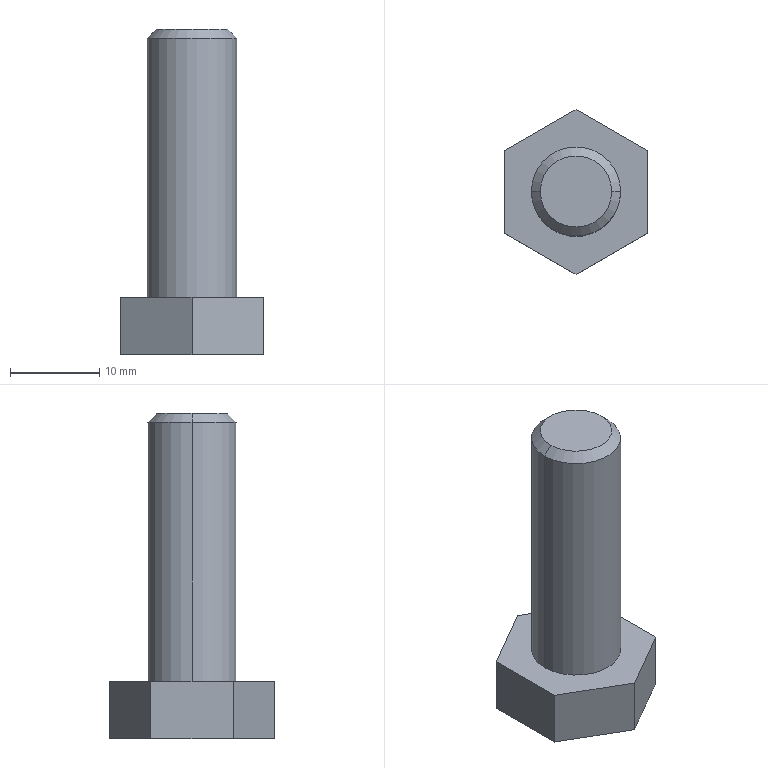Part | SolidWorks | features Chamfer 1, Extrusion 1, ICE 1, RefAxis 1 | 1 solid | 13 faces | box 16 x 18.475 x 36.4 mm | volume 3760 mm3 | plane 9 | cone 2 | cylinder 2 | commonest cylinder face diameters 10 x2
STEP:
#1=CARTESIAN_POINT('',(4.,0.,36.4));
#2=VERTEX_POINT('',#1);
#3=CARTESIAN_POINT('',(-4.,0.,36.4));
#4=VERTEX_POINT('',#3);
#5=CARTESIAN_POINT('',(0.,0.,36.4));
#6=DIRECTION('',(0.,0.,1.));
#7=DIRECTION('',(1.,0.,0.));
#8=AXIS2_PLACEMENT_3D('',#5,#6,#7);
#9=CIRCLE('',#8,4.);
#10=EDGE_CURVE('',#2,#4,#9,.T.);
#11=ORIENTED_EDGE('',*,*,#10,.F.);
#12=CARTESIAN_POINT('',(5.,0.,35.4));
#13=VERTEX_POINT('',#12);
#14=CARTESIAN_POINT('',(4.,0.,36.4));
#15=DIRECTION('',(0.7071,0.,-0.7071));
#16=VECTOR('',#15,1000.);
#17=LINE('',#14,#16);
#18=EDGE_CURVE('',#2,#13,#17,.T.);
#19=ORIENTED_EDGE('',*,*,#18,.T.);
#20=CARTESIAN_POINT('',(-5.,0.,35.4));
#21=VERTEX_POINT('',#20);
#22=CARTESIAN_POINT('',(0.,0.,35.4));
#23=DIRECTION('',(0.,0.,-1.));
#24=DIRECTION('',(1.,0.,0.));
#25=AXIS2_PLACEMENT_3D('',#22,#23,#24);
#26=CIRCLE('',#25,5.);
#27=EDGE_CURVE('',#21,#13,#26,.T.);
#28=ORIENTED_EDGE('',*,*,#27,.F.);
#29=CARTESIAN_POINT('',(-4.,0.,36.4));
#30=DIRECTION('',(-0.7071,0.,-0.7071));
#31=VECTOR('',#30,1000.);
#32=LINE('',#29,#31);
#33=EDGE_CURVE('',#4,#21,#32,.T.);
#34=ORIENTED_EDGE('',*,*,#33,.F.);
#35=EDGE_LOOP('',(#11,#19,#28,#34));
#36=FACE_OUTER_BOUND('',#35,.T.);
#37=CARTESIAN_POINT('',(0.,0.,36.4));
#38=DIRECTION('',(0.,0.,-1.));
#39=DIRECTION('',(-1.,0.,0.));
#40=AXIS2_PLACEMENT_3D('',#37,#38,#39);
#41=CONICAL_SURFACE('',#40,4.,0.7854);
#42=ADVANCED_FACE('',(#36),#41,.T.);
#43=ORIENTED_EDGE('',*,*,#27,.T.);
#44=CARTESIAN_POINT('',(5.,0.,6.4));
#45=VERTEX_POINT('',#44);
#46=CARTESIAN_POINT('',(5.,0.,36.4));
#47=DIRECTION('',(0.,0.,-1.));
#48=VECTOR('',#47,1000.);
#49=LINE('',#46,#48);
#50=EDGE_CURVE('',#13,#45,#49,.T.);
#51=ORIENTED_EDGE('',*,*,#50,.T.);
#52=CARTESIAN_POINT('',(-5.,0.,6.4));
#53=VERTEX_POINT('',#52);
#54=CARTESIAN_POINT('',(0.,0.,6.4));
#55=DIRECTION('',(0.,0.,1.));
#56=DIRECTION('',(1.,0.,0.));
#57=AXIS2_PLACEMENT_3D('',#54,#55,#56);
#58=CIRCLE('',#57,5.);
#59=EDGE_CURVE('',#45,#53,#58,.T.);
#60=ORIENTED_EDGE('',*,*,#59,.T.);
#61=CARTESIAN_POINT('',(-5.,0.,36.4));
#62=DIRECTION('',(0.,0.,-1.));
#63=VECTOR('',#62,1000.);
#64=LINE('',#61,#63);
#65=EDGE_CURVE('',#21,#53,#64,.T.);
#66=ORIENTED_EDGE('',*,*,#65,.F.);
#67=EDGE_LOOP('',(#43,#51,#60,#66));
#68=FACE_OUTER_BOUND('',#67,.T.);
#69=CARTESIAN_POINT('',(0.,0.,36.4));
#70=DIRECTION('',(0.,0.,-1.));
#71=DIRECTION('',(-1.,0.,0.));
#72=AXIS2_PLACEMENT_3D('',#69,#70,#71);
#73=CYLINDRICAL_SURFACE('',#72,5.);
#74=ADVANCED_FACE('',(#68),#73,.T.);
#75=CARTESIAN_POINT('',(8.,-4.619,6.4));
#76=VERTEX_POINT('',#75);
#77=CARTESIAN_POINT('',(8.,4.619,6.4));
#78=VERTEX_POINT('',#77);
#79=CARTESIAN_POINT('',(8.,-4.619,6.4));
#80=DIRECTION('',(0.,1.,0.));
#81=VECTOR('',#80,1000.);
#82=LINE('',#79,#81);
#83=EDGE_CURVE('',#76,#78,#82,.T.);
#84=ORIENTED_EDGE('',*,*,#83,.T.);
#85=CARTESIAN_POINT('',(0.,9.238,6.4));
#86=VERTEX_POINT('',#85);
#87=CARTESIAN_POINT('',(8.,4.619,6.4));
#88=DIRECTION('',(-0.866,0.5,0.));
#89=VECTOR('',#88,1000.);
#90=LINE('',#87,#89);
#91=EDGE_CURVE('',#78,#86,#90,.T.);
#92=ORIENTED_EDGE('',*,*,#91,.T.);
#93=CARTESIAN_POINT('',(-8.,4.619,6.4));
#94=VERTEX_POINT('',#93);
#95=CARTESIAN_POINT('',(0.,9.238,6.4));
#96=DIRECTION('',(-0.866,-0.5,0.));
#97=VECTOR('',#96,1000.);
#98=LINE('',#95,#97);
#99=EDGE_CURVE('',#86,#94,#98,.T.);
#100=ORIENTED_EDGE('',*,*,#99,.T.);
#101=CARTESIAN_POINT('',(-8.,-4.619,6.4));
#102=VERTEX_POINT('',#101);
#103=CARTESIAN_POINT('',(-8.,4.619,6.4));
#104=DIRECTION('',(0.,-1.,0.));
#105=VECTOR('',#104,1000.);
#106=LINE('',#103,#105);
#107=EDGE_CURVE('',#94,#102,#106,.T.);
#108=ORIENTED_EDGE('',*,*,#107,.T.);
#109=CARTESIAN_POINT('',(0.,-9.238,6.4));
#110=VERTEX_POINT('',#109);
#111=CARTESIAN_POINT('',(-8.,-4.619,6.4));
#112=DIRECTION('',(0.866,-0.5,0.));
#113=VECTOR('',#112,1000.);
#114=LINE('',#111,#113);
#115=EDGE_CURVE('',#102,#110,#114,.T.);
#116=ORIENTED_EDGE('',*,*,#115,.T.);
#117=CARTESIAN_POINT('',(0.,-9.238,6.4));
#118=DIRECTION('',(0.866,0.5,0.));
#119=VECTOR('',#118,1000.);
#120=LINE('',#117,#119);
#121=EDGE_CURVE('',#110,#76,#120,.T.);
#122=ORIENTED_EDGE('',*,*,#121,.T.);
#123=EDGE_LOOP('',(#84,#92,#100,#108,#116,#122));
#124=FACE_OUTER_BOUND('',#123,.T.);
#125=CARTESIAN_POINT('',(0.,0.,6.4));
#126=DIRECTION('',(0.,0.,1.));
#127=DIRECTION('',(1.,0.,0.));
#128=AXIS2_PLACEMENT_3D('',#125,#126,#127);
#129=CIRCLE('',#128,5.);
#130=EDGE_CURVE('',#53,#45,#129,.T.);
#131=ORIENTED_EDGE('',*,*,#130,.F.);
#132=ORIENTED_EDGE('',*,*,#59,.F.);
#133=EDGE_LOOP('',(#131,#132));
#134=FACE_BOUND('',#133,.T.);
#135=CARTESIAN_POINT('',(0.,0.,6.4));
#136=DIRECTION('',(0.,0.,1.));
#137=DIRECTION('',(1.,0.,0.));
#138=AXIS2_PLACEMENT_3D('',#135,#136,#137);
#139=PLANE('',#138);
#140=ADVANCED_FACE('',(#124,#134),#139,.T.);
#141=CARTESIAN_POINT('',(8.,-4.619,0.));
#142=VERTEX_POINT('',#141);
#143=CARTESIAN_POINT('',(8.,4.619,0.));
#144=VERTEX_POINT('',#143);
#145=CARTESIAN_POINT('',(8.,-4.619,0.));
#146=DIRECTION('',(0.,1.,0.));
#147=VECTOR('',#146,1000.);
#148=LINE('',#145,#147);
#149=EDGE_CURVE('',#142,#144,#148,.T.);
#150=ORIENTED_EDGE('',*,*,#149,.T.);
#151=CARTESIAN_POINT('',(8.,4.619,6.4));
#152=DIRECTION('',(0.,0.,-1.));
#153=VECTOR('',#152,1000.);
#154=LINE('',#151,#153);
#155=EDGE_CURVE('',#78,#144,#154,.T.);
#156=ORIENTED_EDGE('',*,*,#155,.F.);
#157=ORIENTED_EDGE('',*,*,#83,.F.);
#158=CARTESIAN_POINT('',(8.,-4.619,6.4));
#159=DIRECTION('',(0.,0.,-1.));
#160=VECTOR('',#159,1000.);
#161=LINE('',#158,#160);
#162=EDGE_CURVE('',#76,#142,#161,.T.);
#163=ORIENTED_EDGE('',*,*,#162,.T.);
#164=EDGE_LOOP('',(#150,#156,#157,#163));
#165=FACE_OUTER_BOUND('',#164,.T.);
#166=CARTESIAN_POINT('',(8.,-4.619,6.4));
#167=DIRECTION('',(-1.,0.,0.));
#168=DIRECTION('',(0.,-1.,0.));
#169=AXIS2_PLACEMENT_3D('',#166,#167,#168);
#170=PLANE('',#169);
#171=ADVANCED_FACE('',(#165),#170,.F.);
#172=CARTESIAN_POINT('',(0.,9.238,0.));
#173=VERTEX_POINT('',#172);
#174=CARTESIAN_POINT('',(8.,4.619,0.));
#175=DIRECTION('',(-0.866,0.5,0.));
#176=VECTOR('',#175,1000.);
#177=LINE('',#174,#176);
#178=EDGE_CURVE('',#144,#173,#177,.T.);
#179=ORIENTED_EDGE('',*,*,#178,.T.);
#180=CARTESIAN_POINT('',(0.,9.238,6.4));
#181=DIRECTION('',(0.,0.,-1.));
#182=VECTOR('',#181,1000.);
#183=LINE('',#180,#182);
#184=EDGE_CURVE('',#86,#173,#183,.T.);
#185=ORIENTED_EDGE('',*,*,#184,.F.);
#186=ORIENTED_EDGE('',*,*,#91,.F.);
#187=ORIENTED_EDGE('',*,*,#155,.T.);
#188=EDGE_LOOP('',(#179,#185,#186,#187));
#189=FACE_OUTER_BOUND('',#188,.T.);
#190=CARTESIAN_POINT('',(8.,4.619,6.4));
#191=DIRECTION('',(-0.5,-0.866,0.));
#192=DIRECTION('',(0.866,-0.5,0.));
#193=AXIS2_PLACEMENT_3D('',#190,#191,#192);
#194=PLANE('',#193);
#195=ADVANCED_FACE('',(#189),#194,.F.);
#196=CARTESIAN_POINT('',(-8.,4.619,0.));
#197=VERTEX_POINT('',#196);
#198=CARTESIAN_POINT('',(0.,9.238,0.));
#199=DIRECTION('',(-0.866,-0.5,0.));
#200=VECTOR('',#199,1000.);
#201=LINE('',#198,#200);
#202=EDGE_CURVE('',#173,#197,#201,.T.);
#203=ORIENTED_EDGE('',*,*,#202,.T.);
#204=CARTESIAN_POINT('',(-8.,4.619,6.4));
#205=DIRECTION('',(0.,0.,-1.));
#206=VECTOR('',#205,1000.);
#207=LINE('',#204,#206);
#208=EDGE_CURVE('',#94,#197,#207,.T.);
#209=ORIENTED_EDGE('',*,*,#208,.F.);
#210=ORIENTED_EDGE('',*,*,#99,.F.);
#211=ORIENTED_EDGE('',*,*,#184,.T.);
#212=EDGE_LOOP('',(#203,#209,#210,#211));
#213=FACE_OUTER_BOUND('',#212,.T.);
#214=CARTESIAN_POINT('',(0.,9.238,6.4));
#215=DIRECTION('',(0.5,-0.866,0.));
#216=DIRECTION('',(0.866,0.5,0.));
#217=AXIS2_PLACEMENT_3D('',#214,#215,#216);
#218=PLANE('',#217);
#219=ADVANCED_FACE('',(#213),#218,.F.);
#220=CARTESIAN_POINT('',(-8.,-4.619,0.));
#221=VERTEX_POINT('',#220);
#222=CARTESIAN_POINT('',(-8.,4.619,0.));
#223=DIRECTION('',(0.,-1.,0.));
#224=VECTOR('',#223,1000.);
#225=LINE('',#222,#224);
#226=EDGE_CURVE('',#197,#221,#225,.T.);
#227=ORIENTED_EDGE('',*,*,#226,.T.);
#228=CARTESIAN_POINT('',(-8.,-4.619,6.4));
#229=DIRECTION('',(0.,0.,-1.));
#230=VECTOR('',#229,1000.);
#231=LINE('',#228,#230);
#232=EDGE_CURVE('',#102,#221,#231,.T.);
#233=ORIENTED_EDGE('',*,*,#232,.F.);
#234=ORIENTED_EDGE('',*,*,#107,.F.);
#235=ORIENTED_EDGE('',*,*,#208,.T.);
#236=EDGE_LOOP('',(#227,#233,#234,#235));
#237=FACE_OUTER_BOUND('',#236,.T.);
#238=CARTESIAN_POINT('',(-8.,4.619,6.4));
#239=DIRECTION('',(1.,0.,0.));
#240=DIRECTION('',(0.,1.,0.));
#241=AXIS2_PLACEMENT_3D('',#238,#239,#240);
#242=PLANE('',#241);
#243=ADVANCED_FACE('',(#237),#242,.F.);
#244=CARTESIAN_POINT('',(0.,-9.238,0.));
#245=VERTEX_POINT('',#244);
#246=CARTESIAN_POINT('',(-8.,-4.619,0.));
#247=DIRECTION('',(0.866,-0.5,0.));
#248=VECTOR('',#247,1000.);
#249=LINE('',#246,#248);
#250=EDGE_CURVE('',#221,#245,#249,.T.);
#251=ORIENTED_EDGE('',*,*,#250,.T.);
#252=CARTESIAN_POINT('',(0.,-9.238,6.4));
#253=DIRECTION('',(0.,0.,-1.));
#254=VECTOR('',#253,1000.);
#255=LINE('',#252,#254);
#256=EDGE_CURVE('',#110,#245,#255,.T.);
#257=ORIENTED_EDGE('',*,*,#256,.F.);
#258=ORIENTED_EDGE('',*,*,#115,.F.);
#259=ORIENTED_EDGE('',*,*,#232,.T.);
#260=EDGE_LOOP('',(#251,#257,#258,#259));
#261=FACE_OUTER_BOUND('',#260,.T.);
#262=CARTESIAN_POINT('',(-8.,-4.619,6.4));
#263=DIRECTION('',(0.5,0.866,0.));
#264=DIRECTION('',(-0.866,0.5,0.));
#265=AXIS2_PLACEMENT_3D('',#262,#263,#264);
#266=PLANE('',#265);
#267=ADVANCED_FACE('',(#261),#266,.F.);
#268=CARTESIAN_POINT('',(0.,-9.238,0.));
#269=DIRECTION('',(0.866,0.5,0.));
#270=VECTOR('',#269,1000.);
#271=LINE('',#268,#270);
#272=EDGE_CURVE('',#245,#142,#271,.T.);
#273=ORIENTED_EDGE('',*,*,#272,.T.);
#274=ORIENTED_EDGE('',*,*,#162,.F.);
#275=ORIENTED_EDGE('',*,*,#121,.F.);
#276=ORIENTED_EDGE('',*,*,#256,.T.);
#277=EDGE_LOOP('',(#273,#274,#275,#276));
#278=FACE_OUTER_BOUND('',#277,.T.);
#279=CARTESIAN_POINT('',(0.,-9.238,6.4));
#280=DIRECTION('',(-0.5,0.866,0.));
#281=DIRECTION('',(-0.866,-0.5,0.));
#282=AXIS2_PLACEMENT_3D('',#279,#280,#281);
#283=PLANE('',#282);
#284=ADVANCED_FACE('',(#278),#283,.F.);
#285=ORIENTED_EDGE('',*,*,#149,.F.);
#286=ORIENTED_EDGE('',*,*,#272,.F.);
#287=ORIENTED_EDGE('',*,*,#250,.F.);
#288=ORIENTED_EDGE('',*,*,#226,.F.);
#289=ORIENTED_EDGE('',*,*,#202,.F.);
#290=ORIENTED_EDGE('',*,*,#178,.F.);
#291=EDGE_LOOP('',(#285,#286,#287,#288,#289,#290));
#292=FACE_OUTER_BOUND('',#291,.T.);
#293=CARTESIAN_POINT('',(0.,0.,0.));
#294=DIRECTION('',(0.,0.,1.));
#295=DIRECTION('',(1.,0.,0.));
#296=AXIS2_PLACEMENT_3D('',#293,#294,#295);
#297=PLANE('',#296);
#298=ADVANCED_FACE('',(#292),#297,.F.);
#299=ORIENTED_EDGE('',*,*,#50,.F.);
#300=CARTESIAN_POINT('',(0.,0.,35.4));
#301=DIRECTION('',(0.,0.,-1.));
#302=DIRECTION('',(1.,0.,0.));
#303=AXIS2_PLACEMENT_3D('',#300,#301,#302);
#304=CIRCLE('',#303,5.);
#305=EDGE_CURVE('',#13,#21,#304,.T.);
#306=ORIENTED_EDGE('',*,*,#305,.T.);
#307=ORIENTED_EDGE('',*,*,#65,.T.);
#308=ORIENTED_EDGE('',*,*,#130,.T.);
#309=EDGE_LOOP('',(#299,#306,#307,#308));
#310=FACE_OUTER_BOUND('',#309,.T.);
#311=CARTESIAN_POINT('',(0.,0.,36.4));
#312=DIRECTION('',(0.,0.,-1.));
#313=DIRECTION('',(-1.,0.,0.));
#314=AXIS2_PLACEMENT_3D('',#311,#312,#313);
#315=CYLINDRICAL_SURFACE('',#314,5.);
#316=ADVANCED_FACE('',(#310),#315,.T.);
#317=CARTESIAN_POINT('',(0.,0.,36.4));
#318=DIRECTION('',(0.,0.,1.));
#319=DIRECTION('',(1.,0.,0.));
#320=AXIS2_PLACEMENT_3D('',#317,#318,#319);
#321=CIRCLE('',#320,4.);
#322=EDGE_CURVE('',#4,#2,#321,.T.);
#323=ORIENTED_EDGE('',*,*,#322,.T.);
#324=ORIENTED_EDGE('',*,*,#10,.T.);
#325=EDGE_LOOP('',(#323,#324));
#326=FACE_OUTER_BOUND('',#325,.T.);
#327=CARTESIAN_POINT('',(0.,0.,36.4));
#328=DIRECTION('',(0.,0.,1.));
#329=DIRECTION('',(1.,0.,0.));
#330=AXIS2_PLACEMENT_3D('',#327,#328,#329);
#331=PLANE('',#330);
#332=ADVANCED_FACE('',(#326),#331,.T.);
#333=ORIENTED_EDGE('',*,*,#18,.F.);
#334=ORIENTED_EDGE('',*,*,#322,.F.);
#335=ORIENTED_EDGE('',*,*,#33,.T.);
#336=ORIENTED_EDGE('',*,*,#305,.F.);
#337=EDGE_LOOP('',(#333,#334,#335,#336));
#338=FACE_OUTER_BOUND('',#337,.T.);
#339=CARTESIAN_POINT('',(0.,0.,36.4));
#340=DIRECTION('',(0.,0.,-1.));
#341=DIRECTION('',(-1.,0.,0.));
#342=AXIS2_PLACEMENT_3D('',#339,#340,#341);
#343=CONICAL_SURFACE('',#342,4.,0.7854);
#344=ADVANCED_FACE('',(#338),#343,.T.);
#345=CLOSED_SHELL('',(#42,#74,#140,#171,#195,#219,#243,#267,#284,#298,#316,#332,#344));
#346=MANIFOLD_SOLID_BREP('',#345);
#347=CARTESIAN_POINT('',(0.,0.,0.));
#348=DIRECTION('',(0.,0.,1.));
#349=DIRECTION('',(1.,0.,0.));
#350=AXIS2_PLACEMENT_3D('',#347,#348,#349);
#351=(LENGTH_UNIT()NAMED_UNIT(*)SI_UNIT(.MILLI.,.METRE.));
#352=UNCERTAINTY_MEASURE_WITH_UNIT(LENGTH_MEASURE(0.00001),#351,'','');
#353=(NAMED_UNIT(*)PLANE_ANGLE_UNIT()SI_UNIT($,.RADIAN.));
#354=(NAMED_UNIT(*)SI_UNIT($,.STERADIAN.)SOLID_ANGLE_UNIT());
#355=(GEOMETRIC_REPRESENTATION_CONTEXT(3)GLOBAL_UNCERTAINTY_ASSIGNED_CONTEXT((#352))GLOBAL_UNIT_ASSIGNED_CONTEXT((#351,#353,#354))REPRESENTATION_CONTEXT('',''));
#356=ADVANCED_BREP_SHAPE_REPRESENTATION('',(#346,#350),#355);